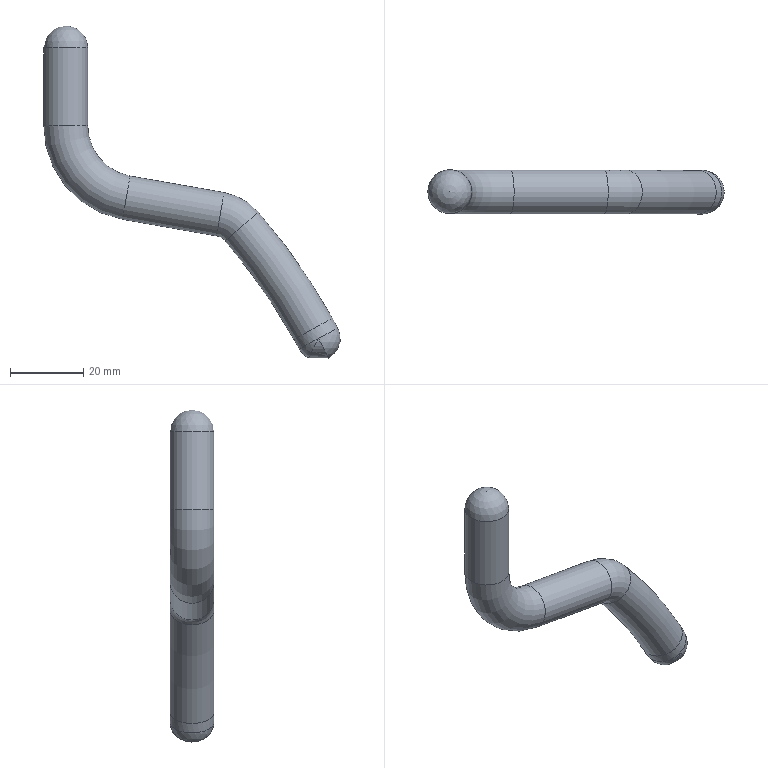Part | STEP file | solid 23 | 1 solid | 11 faces | box 81.042 x 12 x 90.722 mm | volume 14374 mm3 | torus 4 | sphere 3 | cylinder 2 | other 2 | commonest cylinder face diameters 12 x2